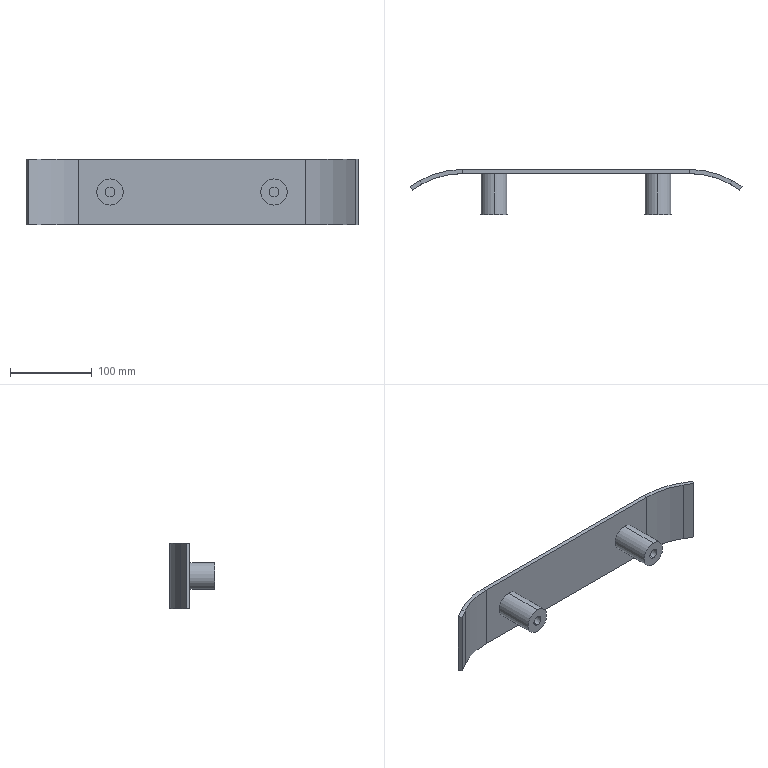Part | SolidWorks | features ICE 2, FlatPattern 1, SMBaseFlange 1, SheetMetal 1 | 1 solid | 34 faces | box 404.961 x 55 x 80 mm | volume 236837 mm3 | plane 22 | cylinder 12 | commonest cylinder face diameters 12 x4 32 x4 200 x2 210 x2
STEP:
#1=CARTESIAN_POINT('',(100.,-15.,6.));
#2=VERTEX_POINT('',#1);
#3=CARTESIAN_POINT('',(100.,-15.,-6.));
#4=VERTEX_POINT('',#3);
#5=CARTESIAN_POINT('',(100.,-15.,0.));
#6=DIRECTION('',(0.,-1.,0.));
#7=DIRECTION('',(0.,0.,-1.));
#8=AXIS2_PLACEMENT_3D('',#5,#6,#7);
#9=CIRCLE('',#8,6.);
#10=EDGE_CURVE('',#2,#4,#9,.T.);
#11=ORIENTED_EDGE('',*,*,#10,.F.);
#12=CARTESIAN_POINT('',(100.,-50.,6.));
#13=VERTEX_POINT('',#12);
#14=CARTESIAN_POINT('',(100.,-15.,6.));
#15=DIRECTION('',(0.,-1.,0.));
#16=VECTOR('',#15,1000.);
#17=LINE('',#14,#16);
#18=EDGE_CURVE('',#2,#13,#17,.T.);
#19=ORIENTED_EDGE('',*,*,#18,.T.);
#20=CARTESIAN_POINT('',(100.,-50.,-6.));
#21=VERTEX_POINT('',#20);
#22=CARTESIAN_POINT('',(100.,-50.,0.));
#23=DIRECTION('',(0.,-1.,0.));
#24=DIRECTION('',(0.,0.,-1.));
#25=AXIS2_PLACEMENT_3D('',#22,#23,#24);
#26=CIRCLE('',#25,6.);
#27=EDGE_CURVE('',#13,#21,#26,.T.);
#28=ORIENTED_EDGE('',*,*,#27,.T.);
#29=CARTESIAN_POINT('',(100.,-15.,-6.));
#30=DIRECTION('',(0.,-1.,0.));
#31=VECTOR('',#30,1000.);
#32=LINE('',#29,#31);
#33=EDGE_CURVE('',#4,#21,#32,.T.);
#34=ORIENTED_EDGE('',*,*,#33,.F.);
#35=EDGE_LOOP('',(#11,#19,#28,#34));
#36=FACE_OUTER_BOUND('',#35,.T.);
#37=CARTESIAN_POINT('',(100.,-15.,0.));
#38=DIRECTION('',(0.,-1.,0.));
#39=DIRECTION('',(0.,0.,-1.));
#40=AXIS2_PLACEMENT_3D('',#37,#38,#39);
#41=CYLINDRICAL_SURFACE('',#40,6.);
#42=ADVANCED_FACE('',(#36),#41,.F.);
#43=CARTESIAN_POINT('',(-100.,-15.,6.));
#44=VERTEX_POINT('',#43);
#45=CARTESIAN_POINT('',(-100.,-15.,-6.));
#46=VERTEX_POINT('',#45);
#47=CARTESIAN_POINT('',(-100.,-15.,0.));
#48=DIRECTION('',(0.,-1.,0.));
#49=DIRECTION('',(0.,0.,-1.));
#50=AXIS2_PLACEMENT_3D('',#47,#48,#49);
#51=CIRCLE('',#50,6.);
#52=EDGE_CURVE('',#44,#46,#51,.T.);
#53=ORIENTED_EDGE('',*,*,#52,.F.);
#54=CARTESIAN_POINT('',(-100.,-50.,6.));
#55=VERTEX_POINT('',#54);
#56=CARTESIAN_POINT('',(-100.,-15.,6.));
#57=DIRECTION('',(0.,-1.,0.));
#58=VECTOR('',#57,1000.);
#59=LINE('',#56,#58);
#60=EDGE_CURVE('',#44,#55,#59,.T.);
#61=ORIENTED_EDGE('',*,*,#60,.T.);
#62=CARTESIAN_POINT('',(-100.,-50.,-6.));
#63=VERTEX_POINT('',#62);
#64=CARTESIAN_POINT('',(-100.,-50.,0.));
#65=DIRECTION('',(0.,-1.,0.));
#66=DIRECTION('',(0.,0.,-1.));
#67=AXIS2_PLACEMENT_3D('',#64,#65,#66);
#68=CIRCLE('',#67,6.);
#69=EDGE_CURVE('',#55,#63,#68,.T.);
#70=ORIENTED_EDGE('',*,*,#69,.T.);
#71=CARTESIAN_POINT('',(-100.,-15.,-6.));
#72=DIRECTION('',(0.,-1.,0.));
#73=VECTOR('',#72,1000.);
#74=LINE('',#71,#73);
#75=EDGE_CURVE('',#46,#63,#74,.T.);
#76=ORIENTED_EDGE('',*,*,#75,.F.);
#77=EDGE_LOOP('',(#53,#61,#70,#76));
#78=FACE_OUTER_BOUND('',#77,.T.);
#79=CARTESIAN_POINT('',(-100.,-15.,0.));
#80=DIRECTION('',(0.,-1.,0.));
#81=DIRECTION('',(0.,0.,-1.));
#82=AXIS2_PLACEMENT_3D('',#79,#80,#81);
#83=CYLINDRICAL_SURFACE('',#82,6.);
#84=ADVANCED_FACE('',(#78),#83,.F.);
#85=CARTESIAN_POINT('',(-100.,-50.,-16.));
#86=VERTEX_POINT('',#85);
#87=CARTESIAN_POINT('',(-100.,-50.,16.));
#88=VERTEX_POINT('',#87);
#89=CARTESIAN_POINT('',(-100.,-50.,0.));
#90=DIRECTION('',(0.,-1.,0.));
#91=DIRECTION('',(0.,0.,-1.));
#92=AXIS2_PLACEMENT_3D('',#89,#90,#91);
#93=CIRCLE('',#92,16.);
#94=EDGE_CURVE('',#86,#88,#93,.T.);
#95=ORIENTED_EDGE('',*,*,#94,.F.);
#96=CARTESIAN_POINT('',(-100.,0.,-16.));
#97=VERTEX_POINT('',#96);
#98=CARTESIAN_POINT('',(-100.,-50.,-16.));
#99=DIRECTION('',(0.,1.,0.));
#100=VECTOR('',#99,1000.);
#101=LINE('',#98,#100);
#102=EDGE_CURVE('',#86,#97,#101,.T.);
#103=ORIENTED_EDGE('',*,*,#102,.T.);
#104=CARTESIAN_POINT('',(-100.,0.,16.));
#105=VERTEX_POINT('',#104);
#106=CARTESIAN_POINT('',(-100.,0.,0.));
#107=DIRECTION('',(0.,-1.,0.));
#108=DIRECTION('',(0.,0.,-1.));
#109=AXIS2_PLACEMENT_3D('',#106,#107,#108);
#110=CIRCLE('',#109,16.);
#111=EDGE_CURVE('',#97,#105,#110,.T.);
#112=ORIENTED_EDGE('',*,*,#111,.T.);
#113=CARTESIAN_POINT('',(-100.,-50.,16.));
#114=DIRECTION('',(0.,1.,0.));
#115=VECTOR('',#114,1000.);
#116=LINE('',#113,#115);
#117=EDGE_CURVE('',#88,#105,#116,.T.);
#118=ORIENTED_EDGE('',*,*,#117,.F.);
#119=EDGE_LOOP('',(#95,#103,#112,#118));
#120=FACE_OUTER_BOUND('',#119,.T.);
#121=CARTESIAN_POINT('',(-100.,-50.,0.));
#122=DIRECTION('',(0.,1.,0.));
#123=DIRECTION('',(0.,0.,1.));
#124=AXIS2_PLACEMENT_3D('',#121,#122,#123);
#125=CYLINDRICAL_SURFACE('',#124,16.);
#126=ADVANCED_FACE('',(#120),#125,.T.);
#127=CARTESIAN_POINT('',(100.,-50.,-16.));
#128=VERTEX_POINT('',#127);
#129=CARTESIAN_POINT('',(100.,-50.,16.));
#130=VERTEX_POINT('',#129);
#131=CARTESIAN_POINT('',(100.,-50.,0.));
#132=DIRECTION('',(0.,-1.,0.));
#133=DIRECTION('',(0.,0.,-1.));
#134=AXIS2_PLACEMENT_3D('',#131,#132,#133);
#135=CIRCLE('',#134,16.);
#136=EDGE_CURVE('',#128,#130,#135,.T.);
#137=ORIENTED_EDGE('',*,*,#136,.F.);
#138=CARTESIAN_POINT('',(100.,0.,-16.));
#139=VERTEX_POINT('',#138);
#140=CARTESIAN_POINT('',(100.,-50.,-16.));
#141=DIRECTION('',(0.,1.,0.));
#142=VECTOR('',#141,1000.);
#143=LINE('',#140,#142);
#144=EDGE_CURVE('',#128,#139,#143,.T.);
#145=ORIENTED_EDGE('',*,*,#144,.T.);
#146=CARTESIAN_POINT('',(100.,0.,16.));
#147=VERTEX_POINT('',#146);
#148=CARTESIAN_POINT('',(100.,0.,0.));
#149=DIRECTION('',(0.,-1.,0.));
#150=DIRECTION('',(0.,0.,-1.));
#151=AXIS2_PLACEMENT_3D('',#148,#149,#150);
#152=CIRCLE('',#151,16.);
#153=EDGE_CURVE('',#139,#147,#152,.T.);
#154=ORIENTED_EDGE('',*,*,#153,.T.);
#155=CARTESIAN_POINT('',(100.,-50.,16.));
#156=DIRECTION('',(0.,1.,0.));
#157=VECTOR('',#156,1000.);
#158=LINE('',#155,#157);
#159=EDGE_CURVE('',#130,#147,#158,.T.);
#160=ORIENTED_EDGE('',*,*,#159,.F.);
#161=EDGE_LOOP('',(#137,#145,#154,#160));
#162=FACE_OUTER_BOUND('',#161,.T.);
#163=CARTESIAN_POINT('',(100.,-50.,0.));
#164=DIRECTION('',(0.,1.,0.));
#165=DIRECTION('',(0.,0.,1.));
#166=AXIS2_PLACEMENT_3D('',#163,#164,#165);
#167=CYLINDRICAL_SURFACE('',#166,16.);
#168=ADVANCED_FACE('',(#162),#167,.T.);
#169=CARTESIAN_POINT('',(138.444,0.,40.));
#170=VERTEX_POINT('',#169);
#171=CARTESIAN_POINT('',(138.444,5.,40.));
#172=VERTEX_POINT('',#171);
#173=CARTESIAN_POINT('',(138.444,0.,40.));
#174=DIRECTION('',(0.,1.,0.));
#175=VECTOR('',#174,1000.);
#176=LINE('',#173,#175);
#177=EDGE_CURVE('',#170,#172,#176,.T.);
#178=ORIENTED_EDGE('',*,*,#177,.F.);
#179=CARTESIAN_POINT('',(188.057,-13.176,40.));
#180=VERTEX_POINT('',#179);
#181=CARTESIAN_POINT('',(138.444,-100.,40.));
#182=DIRECTION('',(0.,0.,1.));
#183=DIRECTION('',(-1.,0.,0.));
#184=AXIS2_PLACEMENT_3D('',#181,#182,#183);
#185=CIRCLE('',#184,100.);
#186=EDGE_CURVE('',#180,#170,#185,.T.);
#187=ORIENTED_EDGE('',*,*,#186,.F.);
#188=CARTESIAN_POINT('',(190.538,-8.834,40.));
#189=VERTEX_POINT('',#188);
#190=CARTESIAN_POINT('',(190.538,-8.834,40.));
#191=DIRECTION('',(-0.4961,-0.8682,0.));
#192=VECTOR('',#191,1000.);
#193=LINE('',#190,#192);
#194=EDGE_CURVE('',#189,#180,#193,.T.);
#195=ORIENTED_EDGE('',*,*,#194,.F.);
#196=CARTESIAN_POINT('',(138.444,-100.,40.));
#197=DIRECTION('',(0.,0.,1.));
#198=DIRECTION('',(1.,0.,0.));
#199=AXIS2_PLACEMENT_3D('',#196,#197,#198);
#200=CIRCLE('',#199,105.);
#201=EDGE_CURVE('',#189,#172,#200,.T.);
#202=ORIENTED_EDGE('',*,*,#201,.T.);
#203=EDGE_LOOP('',(#178,#187,#195,#202));
#204=FACE_OUTER_BOUND('',#203,.T.);
#205=CARTESIAN_POINT('',(138.444,0.,40.));
#206=DIRECTION('',(0.,0.,1.));
#207=DIRECTION('',(1.,0.,0.));
#208=AXIS2_PLACEMENT_3D('',#205,#206,#207);
#209=PLANE('',#208);
#210=ADVANCED_FACE('',(#204),#209,.T.);
#211=CARTESIAN_POINT('',(-138.444,0.,40.));
#212=VERTEX_POINT('',#211);
#213=CARTESIAN_POINT('',(-165.,0.,40.));
#214=DIRECTION('',(-1.,0.,0.));
#215=VECTOR('',#214,1000.);
#216=LINE('',#213,#215);
#217=EDGE_CURVE('',#170,#212,#216,.T.);
#218=ORIENTED_EDGE('',*,*,#217,.F.);
#219=ORIENTED_EDGE('',*,*,#177,.T.);
#220=CARTESIAN_POINT('',(-138.444,5.,40.));
#221=VERTEX_POINT('',#220);
#222=CARTESIAN_POINT('',(-165.,5.,40.));
#223=DIRECTION('',(-1.,0.,0.));
#224=VECTOR('',#223,1000.);
#225=LINE('',#222,#224);
#226=EDGE_CURVE('',#172,#221,#225,.T.);
#227=ORIENTED_EDGE('',*,*,#226,.T.);
#228=CARTESIAN_POINT('',(-138.444,5.,40.));
#229=DIRECTION('',(0.,-1.,0.));
#230=VECTOR('',#229,1000.);
#231=LINE('',#228,#230);
#232=EDGE_CURVE('',#221,#212,#231,.T.);
#233=ORIENTED_EDGE('',*,*,#232,.T.);
#234=EDGE_LOOP('',(#218,#219,#227,#233));
#235=FACE_OUTER_BOUND('',#234,.T.);
#236=CARTESIAN_POINT('',(190.538,-8.834,40.));
#237=DIRECTION('',(0.,0.,1.));
#238=DIRECTION('',(1.,0.,0.));
#239=AXIS2_PLACEMENT_3D('',#236,#237,#238);
#240=PLANE('',#239);
#241=ADVANCED_FACE('',(#235),#240,.T.);
#242=CARTESIAN_POINT('',(188.057,-13.176,-40.));
#243=VERTEX_POINT('',#242);
#244=CARTESIAN_POINT('',(190.538,-8.834,-40.));
#245=VERTEX_POINT('',#244);
#246=CARTESIAN_POINT('',(188.057,-13.176,-40.));
#247=DIRECTION('',(0.4961,0.8682,0.));
#248=VECTOR('',#247,1000.);
#249=LINE('',#246,#248);
#250=EDGE_CURVE('',#243,#245,#249,.T.);
#251=ORIENTED_EDGE('',*,*,#250,.F.);
#252=CARTESIAN_POINT('',(138.444,0.,-40.));
#253=VERTEX_POINT('',#252);
#254=CARTESIAN_POINT('',(138.444,-100.,-40.));
#255=DIRECTION('',(0.,0.,1.));
#256=DIRECTION('',(-1.,0.,0.));
#257=AXIS2_PLACEMENT_3D('',#254,#255,#256);
#258=CIRCLE('',#257,100.);
#259=EDGE_CURVE('',#243,#253,#258,.T.);
#260=ORIENTED_EDGE('',*,*,#259,.T.);
#261=CARTESIAN_POINT('',(138.444,5.,-40.));
#262=VERTEX_POINT('',#261);
#263=CARTESIAN_POINT('',(138.444,5.,-40.));
#264=DIRECTION('',(0.,-1.,0.));
#265=VECTOR('',#264,1000.);
#266=LINE('',#263,#265);
#267=EDGE_CURVE('',#262,#253,#266,.T.);
#268=ORIENTED_EDGE('',*,*,#267,.F.);
#269=CARTESIAN_POINT('',(138.444,-100.,-40.));
#270=DIRECTION('',(0.,0.,1.));
#271=DIRECTION('',(1.,0.,0.));
#272=AXIS2_PLACEMENT_3D('',#269,#270,#271);
#273=CIRCLE('',#272,105.);
#274=EDGE_CURVE('',#245,#262,#273,.T.);
#275=ORIENTED_EDGE('',*,*,#274,.F.);
#276=EDGE_LOOP('',(#251,#260,#268,#275));
#277=FACE_OUTER_BOUND('',#276,.T.);
#278=CARTESIAN_POINT('',(188.057,-13.176,-40.));
#279=DIRECTION('',(0.,0.,-1.));
#280=DIRECTION('',(-1.,0.,0.));
#281=AXIS2_PLACEMENT_3D('',#278,#279,#280);
#282=PLANE('',#281);
#283=ADVANCED_FACE('',(#277),#282,.T.);
#284=CARTESIAN_POINT('',(200.,-20.,-40.));
#285=VERTEX_POINT('',#284);
#286=CARTESIAN_POINT('',(165.,0.,-40.));
#287=DIRECTION('',(-0.8682,0.4961,0.));
#288=VECTOR('',#287,1000.);
#289=LINE('',#286,#288);
#290=EDGE_CURVE('',#285,#243,#289,.T.);
#291=ORIENTED_EDGE('',*,*,#290,.T.);
#292=ORIENTED_EDGE('',*,*,#250,.T.);
#293=CARTESIAN_POINT('',(202.481,-15.659,-40.));
#294=VERTEX_POINT('',#293);
#295=CARTESIAN_POINT('',(167.481,4.341,-40.));
#296=DIRECTION('',(-0.8682,0.4961,0.));
#297=VECTOR('',#296,1000.);
#298=LINE('',#295,#297);
#299=EDGE_CURVE('',#294,#245,#298,.T.);
#300=ORIENTED_EDGE('',*,*,#299,.F.);
#301=CARTESIAN_POINT('',(202.481,-15.659,-40.));
#302=DIRECTION('',(-0.4961,-0.8682,0.));
#303=VECTOR('',#302,1000.);
#304=LINE('',#301,#303);
#305=EDGE_CURVE('',#294,#285,#304,.T.);
#306=ORIENTED_EDGE('',*,*,#305,.T.);
#307=EDGE_LOOP('',(#291,#292,#300,#306));
#308=FACE_OUTER_BOUND('',#307,.T.);
#309=CARTESIAN_POINT('',(138.444,5.,-40.));
#310=DIRECTION('',(0.,0.,-1.));
#311=DIRECTION('',(-1.,0.,0.));
#312=AXIS2_PLACEMENT_3D('',#309,#310,#311);
#313=PLANE('',#312);
#314=ADVANCED_FACE('',(#308),#313,.T.);
#315=CARTESIAN_POINT('',(-188.057,-13.176,40.));
#316=VERTEX_POINT('',#315);
#317=CARTESIAN_POINT('',(-190.538,-8.834,40.));
#318=VERTEX_POINT('',#317);
#319=CARTESIAN_POINT('',(-188.057,-13.176,40.));
#320=DIRECTION('',(-0.4961,0.8682,0.));
#321=VECTOR('',#320,1000.);
#322=LINE('',#319,#321);
#323=EDGE_CURVE('',#316,#318,#322,.T.);
#324=ORIENTED_EDGE('',*,*,#323,.F.);
#325=CARTESIAN_POINT('',(-138.444,-100.,40.));
#326=DIRECTION('',(0.,0.,1.));
#327=DIRECTION('',(-1.,0.,0.));
#328=AXIS2_PLACEMENT_3D('',#325,#326,#327);
#329=CIRCLE('',#328,100.);
#330=EDGE_CURVE('',#212,#316,#329,.T.);
#331=ORIENTED_EDGE('',*,*,#330,.F.);
#332=ORIENTED_EDGE('',*,*,#232,.F.);
#333=CARTESIAN_POINT('',(-138.444,-100.,40.));
#334=DIRECTION('',(0.,0.,1.));
#335=DIRECTION('',(1.,0.,0.));
#336=AXIS2_PLACEMENT_3D('',#333,#334,#335);
#337=CIRCLE('',#336,105.);
#338=EDGE_CURVE('',#221,#318,#337,.T.);
#339=ORIENTED_EDGE('',*,*,#338,.T.);
#340=EDGE_LOOP('',(#324,#331,#332,#339));
#341=FACE_OUTER_BOUND('',#340,.T.);
#342=CARTESIAN_POINT('',(-188.057,-13.176,40.));
#343=DIRECTION('',(0.,0.,1.));
#344=DIRECTION('',(1.,0.,0.));
#345=AXIS2_PLACEMENT_3D('',#342,#343,#344);
#346=PLANE('',#345);
#347=ADVANCED_FACE('',(#341),#346,.T.);
#348=CARTESIAN_POINT('',(-200.,-20.,40.));
#349=VERTEX_POINT('',#348);
#350=CARTESIAN_POINT('',(-165.,0.,40.));
#351=DIRECTION('',(-0.8682,-0.4961,0.));
#352=VECTOR('',#351,1000.);
#353=LINE('',#350,#352);
#354=EDGE_CURVE('',#316,#349,#353,.T.);
#355=ORIENTED_EDGE('',*,*,#354,.F.);
#356=ORIENTED_EDGE('',*,*,#323,.T.);
#357=CARTESIAN_POINT('',(-202.481,-15.659,40.));
#358=VERTEX_POINT('',#357);
#359=CARTESIAN_POINT('',(-167.481,4.341,40.));
#360=DIRECTION('',(-0.8682,-0.4961,0.));
#361=VECTOR('',#360,1000.);
#362=LINE('',#359,#361);
#363=EDGE_CURVE('',#318,#358,#362,.T.);
#364=ORIENTED_EDGE('',*,*,#363,.T.);
#365=CARTESIAN_POINT('',(-200.,-20.,40.));
#366=DIRECTION('',(-0.4961,0.8682,0.));
#367=VECTOR('',#366,1000.);
#368=LINE('',#365,#367);
#369=EDGE_CURVE('',#349,#358,#368,.T.);
#370=ORIENTED_EDGE('',*,*,#369,.F.);
#371=EDGE_LOOP('',(#355,#356,#364,#370));
#372=FACE_OUTER_BOUND('',#371,.T.);
#373=CARTESIAN_POINT('',(-138.444,5.,40.));
#374=DIRECTION('',(0.,0.,1.));
#375=DIRECTION('',(1.,0.,0.));
#376=AXIS2_PLACEMENT_3D('',#373,#374,#375);
#377=PLANE('',#376);
#378=ADVANCED_FACE('',(#372),#377,.T.);
#379=CARTESIAN_POINT('',(-138.444,0.,-40.));
#380=VERTEX_POINT('',#379);
#381=CARTESIAN_POINT('',(-138.444,5.,-40.));
#382=VERTEX_POINT('',#381);
#383=CARTESIAN_POINT('',(-138.444,0.,-40.));
#384=DIRECTION('',(0.,1.,0.));
#385=VECTOR('',#384,1000.);
#386=LINE('',#383,#385);
#387=EDGE_CURVE('',#380,#382,#386,.T.);
#388=ORIENTED_EDGE('',*,*,#387,.F.);
#389=CARTESIAN_POINT('',(-188.057,-13.176,-40.));
#390=VERTEX_POINT('',#389);
#391=CARTESIAN_POINT('',(-138.444,-100.,-40.));
#392=DIRECTION('',(0.,0.,1.));
#393=DIRECTION('',(-1.,0.,0.));
#394=AXIS2_PLACEMENT_3D('',#391,#392,#393);
#395=CIRCLE('',#394,100.);
#396=EDGE_CURVE('',#380,#390,#395,.T.);
#397=ORIENTED_EDGE('',*,*,#396,.T.);
#398=CARTESIAN_POINT('',(-190.538,-8.834,-40.));
#399=VERTEX_POINT('',#398);
#400=CARTESIAN_POINT('',(-190.538,-8.834,-40.));
#401=DIRECTION('',(0.4961,-0.8682,0.));
#402=VECTOR('',#401,1000.);
#403=LINE('',#400,#402);
#404=EDGE_CURVE('',#399,#390,#403,.T.);
#405=ORIENTED_EDGE('',*,*,#404,.F.);
#406=CARTESIAN_POINT('',(-138.444,-100.,-40.));
#407=DIRECTION('',(0.,0.,1.));
#408=DIRECTION('',(1.,0.,0.));
#409=AXIS2_PLACEMENT_3D('',#406,#407,#408);
#410=CIRCLE('',#409,105.);
#411=EDGE_CURVE('',#382,#399,#410,.T.);
#412=ORIENTED_EDGE('',*,*,#411,.F.);
#413=EDGE_LOOP('',(#388,#397,#405,#412));
#414=FACE_OUTER_BOUND('',#413,.T.);
#415=CARTESIAN_POINT('',(-138.444,0.,-40.));
#416=DIRECTION('',(0.,0.,-1.));
#417=DIRECTION('',(-1.,0.,0.));
#418=AXIS2_PLACEMENT_3D('',#415,#416,#417);
#419=PLANE('',#418);
#420=ADVANCED_FACE('',(#414),#419,.T.);
#421=CARTESIAN_POINT('',(-165.,0.,-40.));
#422=DIRECTION('',(-1.,0.,0.));
#423=VECTOR('',#422,1000.);
#424=LINE('',#421,#423);
#425=EDGE_CURVE('',#253,#380,#424,.T.);
#426=ORIENTED_EDGE('',*,*,#425,.T.);
#427=ORIENTED_EDGE('',*,*,#387,.T.);
#428=CARTESIAN_POINT('',(-165.,5.,-40.));
#429=DIRECTION('',(-1.,0.,0.));
#430=VECTOR('',#429,1000.);
#431=LINE('',#428,#430);
#432=EDGE_CURVE('',#262,#382,#431,.T.);
#433=ORIENTED_EDGE('',*,*,#432,.F.);
#434=ORIENTED_EDGE('',*,*,#267,.T.);
#435=EDGE_LOOP('',(#426,#427,#433,#434));
#436=FACE_OUTER_BOUND('',#435,.T.);
#437=CARTESIAN_POINT('',(-190.538,-8.834,-40.));
#438=DIRECTION('',(0.,0.,-1.));
#439=DIRECTION('',(-1.,0.,0.));
#440=AXIS2_PLACEMENT_3D('',#437,#438,#439);
#441=PLANE('',#440);
#442=ADVANCED_FACE('',(#436),#441,.T.);
#443=CARTESIAN_POINT('',(-202.481,-15.659,-40.));
#444=VERTEX_POINT('',#443);
#445=CARTESIAN_POINT('',(-167.481,4.341,-40.));
#446=DIRECTION('',(-0.8682,-0.4961,0.));
#447=VECTOR('',#446,1000.);
#448=LINE('',#445,#447);
#449=EDGE_CURVE('',#399,#444,#448,.T.);
#450=ORIENTED_EDGE('',*,*,#449,.T.);
#451=CARTESIAN_POINT('',(-202.481,-15.659,40.));
#452=DIRECTION('',(0.,0.,-1.));
#453=VECTOR('',#452,1000.);
#454=LINE('',#451,#453);
#455=EDGE_CURVE('',#358,#444,#454,.T.);
#456=ORIENTED_EDGE('',*,*,#455,.F.);
#457=ORIENTED_EDGE('',*,*,#363,.F.);
#458=CARTESIAN_POINT('',(-190.538,-8.834,40.));
#459=DIRECTION('',(0.,0.,-1.));
#460=VECTOR('',#459,1000.);
#461=LINE('',#458,#460);
#462=EDGE_CURVE('',#318,#399,#461,.T.);
#463=ORIENTED_EDGE('',*,*,#462,.T.);
#464=EDGE_LOOP('',(#450,#456,#457,#463));
#465=FACE_OUTER_BOUND('',#464,.T.);
#466=CARTESIAN_POINT('',(-167.481,4.341,40.));
#467=DIRECTION('',(0.4961,-0.8682,0.));
#468=DIRECTION('',(0.8682,0.4961,0.));
#469=AXIS2_PLACEMENT_3D('',#466,#467,#468);
#470=PLANE('',#469);
#471=ADVANCED_FACE('',(#465),#470,.F.);
#472=CARTESIAN_POINT('',(-200.,-20.,-40.));
#473=VERTEX_POINT('',#472);
#474=CARTESIAN_POINT('',(-200.,-20.,-40.));
#475=DIRECTION('',(-0.4961,0.8682,0.));
#476=VECTOR('',#475,1000.);
#477=LINE('',#474,#476);
#478=EDGE_CURVE('',#473,#444,#477,.T.);
#479=ORIENTED_EDGE('',*,*,#478,.F.);
#480=CARTESIAN_POINT('',(-200.,-20.,40.));
#481=DIRECTION('',(0.,0.,-1.));
#482=VECTOR('',#481,1000.);
#483=LINE('',#480,#482);
#484=EDGE_CURVE('',#349,#473,#483,.T.);
#485=ORIENTED_EDGE('',*,*,#484,.F.);
#486=ORIENTED_EDGE('',*,*,#369,.T.);
#487=ORIENTED_EDGE('',*,*,#455,.T.);
#488=EDGE_LOOP('',(#479,#485,#486,#487));
#489=FACE_OUTER_BOUND('',#488,.T.);
#490=CARTESIAN_POINT('',(-200.,-20.,40.));
#491=DIRECTION('',(-0.8682,-0.4961,0.));
#492=DIRECTION('',(0.4961,-0.8682,0.));
#493=AXIS2_PLACEMENT_3D('',#490,#491,#492);
#494=PLANE('',#493);
#495=ADVANCED_FACE('',(#489),#494,.T.);
#496=CARTESIAN_POINT('',(-165.,0.,-40.));
#497=DIRECTION('',(-0.8682,-0.4961,0.));
#498=VECTOR('',#497,1000.);
#499=LINE('',#496,#498);
#500=EDGE_CURVE('',#390,#473,#499,.T.);
#501=ORIENTED_EDGE('',*,*,#500,.F.);
#502=CARTESIAN_POINT('',(-188.057,-13.176,40.));
#503=DIRECTION('',(0.,0.,-1.));
#504=VECTOR('',#503,1000.);
#505=LINE('',#502,#504);
#506=EDGE_CURVE('',#316,#390,#505,.T.);
#507=ORIENTED_EDGE('',*,*,#506,.F.);
#508=ORIENTED_EDGE('',*,*,#354,.T.);
#509=ORIENTED_EDGE('',*,*,#484,.T.);
#510=EDGE_LOOP('',(#501,#507,#508,#509));
#511=FACE_OUTER_BOUND('',#510,.T.);
#512=CARTESIAN_POINT('',(-165.,0.,40.));
#513=DIRECTION('',(0.4961,-0.8682,0.));
#514=DIRECTION('',(0.8682,0.4961,0.));
#515=AXIS2_PLACEMENT_3D('',#512,#513,#514);
#516=PLANE('',#515);
#517=ADVANCED_FACE('',(#511),#516,.T.);
#518=ORIENTED_EDGE('',*,*,#396,.F.);
#519=CARTESIAN_POINT('',(-138.444,0.,40.));
#520=DIRECTION('',(0.,0.,-1.));
#521=VECTOR('',#520,1000.);
#522=LINE('',#519,#521);
#523=EDGE_CURVE('',#212,#380,#522,.T.);
#524=ORIENTED_EDGE('',*,*,#523,.F.);
#525=ORIENTED_EDGE('',*,*,#330,.T.);
#526=ORIENTED_EDGE('',*,*,#506,.T.);
#527=EDGE_LOOP('',(#518,#524,#525,#526));
#528=FACE_OUTER_BOUND('',#527,.T.);
#529=CARTESIAN_POINT('',(-138.444,-100.,40.));
#530=DIRECTION('',(0.,0.,-1.));
#531=DIRECTION('',(-1.,0.,0.));
#532=AXIS2_PLACEMENT_3D('',#529,#530,#531);
#533=CYLINDRICAL_SURFACE('',#532,100.);
#534=ADVANCED_FACE('',(#528),#533,.F.);
#535=CARTESIAN_POINT('',(-100.,0.,0.));
#536=DIRECTION('',(0.,-1.,0.));
#537=DIRECTION('',(0.,0.,-1.));
#538=AXIS2_PLACEMENT_3D('',#535,#536,#537);
#539=CIRCLE('',#538,16.);
#540=EDGE_CURVE('',#105,#97,#539,.T.);
#541=ORIENTED_EDGE('',*,*,#540,.F.);
#542=ORIENTED_EDGE('',*,*,#111,.F.);
#543=EDGE_LOOP('',(#541,#542));
#544=FACE_BOUND('',#543,.T.);
#545=CARTESIAN_POINT('',(100.,0.,0.));
#546=DIRECTION('',(0.,-1.,0.));
#547=DIRECTION('',(0.,0.,-1.));
#548=AXIS2_PLACEMENT_3D('',#545,#546,#547);
#549=CIRCLE('',#548,16.);
#550=EDGE_CURVE('',#147,#139,#549,.T.);
#551=ORIENTED_EDGE('',*,*,#550,.F.);
#552=ORIENTED_EDGE('',*,*,#153,.F.);
#553=EDGE_LOOP('',(#551,#552));
#554=FACE_BOUND('',#553,.T.);
#555=ORIENTED_EDGE('',*,*,#425,.F.);
#556=CARTESIAN_POINT('',(138.444,0.,40.));
#557=DIRECTION('',(0.,0.,-1.));
#558=VECTOR('',#557,1000.);
#559=LINE('',#556,#558);
#560=EDGE_CURVE('',#170,#253,#559,.T.);
#561=ORIENTED_EDGE('',*,*,#560,.F.);
#562=ORIENTED_EDGE('',*,*,#217,.T.);
#563=ORIENTED_EDGE('',*,*,#523,.T.);
#564=EDGE_LOOP('',(#555,#561,#562,#563));
#565=FACE_OUTER_BOUND('',#564,.T.);
#566=CARTESIAN_POINT('',(-165.,0.,40.));
#567=DIRECTION('',(0.,-1.,0.));
#568=DIRECTION('',(0.,0.,-1.));
#569=AXIS2_PLACEMENT_3D('',#566,#567,#568);
#570=PLANE('',#569);
#571=ADVANCED_FACE('',(#544,#554,#565),#570,.T.);
#572=ORIENTED_EDGE('',*,*,#259,.F.);
#573=CARTESIAN_POINT('',(188.057,-13.176,40.));
#574=DIRECTION('',(0.,0.,-1.));
#575=VECTOR('',#574,1000.);
#576=LINE('',#573,#575);
#577=EDGE_CURVE('',#180,#243,#576,.T.);
#578=ORIENTED_EDGE('',*,*,#577,.F.);
#579=ORIENTED_EDGE('',*,*,#186,.T.);
#580=ORIENTED_EDGE('',*,*,#560,.T.);
#581=EDGE_LOOP('',(#572,#578,#579,#580));
#582=FACE_OUTER_BOUND('',#581,.T.);
#583=CARTESIAN_POINT('',(138.444,-100.,40.));
#584=DIRECTION('',(0.,0.,-1.));
#585=DIRECTION('',(-1.,0.,0.));
#586=AXIS2_PLACEMENT_3D('',#583,#584,#585);
#587=CYLINDRICAL_SURFACE('',#586,100.);
#588=ADVANCED_FACE('',(#582),#587,.F.);
#589=ORIENTED_EDGE('',*,*,#290,.F.);
#590=CARTESIAN_POINT('',(200.,-20.,40.));
#591=VERTEX_POINT('',#590);
#592=CARTESIAN_POINT('',(200.,-20.,40.));
#593=DIRECTION('',(0.,0.,-1.));
#594=VECTOR('',#593,1000.);
#595=LINE('',#592,#594);
#596=EDGE_CURVE('',#591,#285,#595,.T.);
#597=ORIENTED_EDGE('',*,*,#596,.F.);
#598=CARTESIAN_POINT('',(165.,0.,40.));
#599=DIRECTION('',(-0.8682,0.4961,0.));
#600=VECTOR('',#599,1000.);
#601=LINE('',#598,#600);
#602=EDGE_CURVE('',#591,#180,#601,.T.);
#603=ORIENTED_EDGE('',*,*,#602,.T.);
#604=ORIENTED_EDGE('',*,*,#577,.T.);
#605=EDGE_LOOP('',(#589,#597,#603,#604));
#606=FACE_OUTER_BOUND('',#605,.T.);
#607=CARTESIAN_POINT('',(165.,0.,40.));
#608=DIRECTION('',(-0.4961,-0.8682,0.));
#609=DIRECTION('',(0.8682,-0.4961,0.));
#610=AXIS2_PLACEMENT_3D('',#607,#608,#609);
#611=PLANE('',#610);
#612=ADVANCED_FACE('',(#606),#611,.T.);
#613=ORIENTED_EDGE('',*,*,#305,.F.);
#614=CARTESIAN_POINT('',(202.481,-15.659,40.));
#615=VERTEX_POINT('',#614);
#616=CARTESIAN_POINT('',(202.481,-15.659,40.));
#617=DIRECTION('',(0.,0.,-1.));
#618=VECTOR('',#617,1000.);
#619=LINE('',#616,#618);
#620=EDGE_CURVE('',#615,#294,#619,.T.);
#621=ORIENTED_EDGE('',*,*,#620,.F.);
#622=CARTESIAN_POINT('',(202.481,-15.659,40.));
#623=DIRECTION('',(-0.4961,-0.8682,0.));
#624=VECTOR('',#623,1000.);
#625=LINE('',#622,#624);
#626=EDGE_CURVE('',#615,#591,#625,.T.);
#627=ORIENTED_EDGE('',*,*,#626,.T.);
#628=ORIENTED_EDGE('',*,*,#596,.T.);
#629=EDGE_LOOP('',(#613,#621,#627,#628));
#630=FACE_OUTER_BOUND('',#629,.T.);
#631=CARTESIAN_POINT('',(202.481,-15.659,40.));
#632=DIRECTION('',(0.8682,-0.4961,0.));
#633=DIRECTION('',(0.4961,0.8682,0.));
#634=AXIS2_PLACEMENT_3D('',#631,#632,#633);
#635=PLANE('',#634);
#636=ADVANCED_FACE('',(#630),#635,.T.);
#637=ORIENTED_EDGE('',*,*,#299,.T.);
#638=CARTESIAN_POINT('',(190.538,-8.834,40.));
#639=DIRECTION('',(0.,0.,-1.));
#640=VECTOR('',#639,1000.);
#641=LINE('',#638,#640);
#642=EDGE_CURVE('',#189,#245,#641,.T.);
#643=ORIENTED_EDGE('',*,*,#642,.F.);
#644=CARTESIAN_POINT('',(167.481,4.341,40.));
#645=DIRECTION('',(-0.8682,0.4961,0.));
#646=VECTOR('',#645,1000.);
#647=LINE('',#644,#646);
#648=EDGE_CURVE('',#615,#189,#647,.T.);
#649=ORIENTED_EDGE('',*,*,#648,.F.);
#650=ORIENTED_EDGE('',*,*,#620,.T.);
#651=EDGE_LOOP('',(#637,#643,#649,#650));
#652=FACE_OUTER_BOUND('',#651,.T.);
#653=CARTESIAN_POINT('',(167.481,4.341,40.));
#654=DIRECTION('',(-0.4961,-0.8682,0.));
#655=DIRECTION('',(0.8682,-0.4961,0.));
#656=AXIS2_PLACEMENT_3D('',#653,#654,#655);
#657=PLANE('',#656);
#658=ADVANCED_FACE('',(#652),#657,.F.);
#659=ORIENTED_EDGE('',*,*,#274,.T.);
#660=CARTESIAN_POINT('',(138.444,5.,40.));
#661=DIRECTION('',(0.,0.,-1.));
#662=VECTOR('',#661,1000.);
#663=LINE('',#660,#662);
#664=EDGE_CURVE('',#172,#262,#663,.T.);
#665=ORIENTED_EDGE('',*,*,#664,.F.);
#666=ORIENTED_EDGE('',*,*,#201,.F.);
#667=ORIENTED_EDGE('',*,*,#642,.T.);
#668=EDGE_LOOP('',(#659,#665,#666,#667));
#669=FACE_OUTER_BOUND('',#668,.T.);
#670=CARTESIAN_POINT('',(138.444,-100.,40.));
#671=DIRECTION('',(0.,0.,-1.));
#672=DIRECTION('',(-1.,0.,0.));
#673=AXIS2_PLACEMENT_3D('',#670,#671,#672);
#674=CYLINDRICAL_SURFACE('',#673,105.);
#675=ADVANCED_FACE('',(#669),#674,.T.);
#676=ORIENTED_EDGE('',*,*,#432,.T.);
#677=CARTESIAN_POINT('',(-138.444,5.,40.));
#678=DIRECTION('',(0.,0.,-1.));
#679=VECTOR('',#678,1000.);
#680=LINE('',#677,#679);
#681=EDGE_CURVE('',#221,#382,#680,.T.);
#682=ORIENTED_EDGE('',*,*,#681,.F.);
#683=ORIENTED_EDGE('',*,*,#226,.F.);
#684=ORIENTED_EDGE('',*,*,#664,.T.);
#685=EDGE_LOOP('',(#676,#682,#683,#684));
#686=FACE_OUTER_BOUND('',#685,.T.);
#687=CARTESIAN_POINT('',(-165.,5.,40.));
#688=DIRECTION('',(0.,-1.,0.));
#689=DIRECTION('',(0.,0.,-1.));
#690=AXIS2_PLACEMENT_3D('',#687,#688,#689);
#691=PLANE('',#690);
#692=ADVANCED_FACE('',(#686),#691,.F.);
#693=ORIENTED_EDGE('',*,*,#411,.T.);
#694=ORIENTED_EDGE('',*,*,#462,.F.);
#695=ORIENTED_EDGE('',*,*,#338,.F.);
#696=ORIENTED_EDGE('',*,*,#681,.T.);
#697=EDGE_LOOP('',(#693,#694,#695,#696));
#698=FACE_OUTER_BOUND('',#697,.T.);
#699=CARTESIAN_POINT('',(-138.444,-100.,40.));
#700=DIRECTION('',(0.,0.,-1.));
#701=DIRECTION('',(-1.,0.,0.));
#702=AXIS2_PLACEMENT_3D('',#699,#700,#701);
#703=CYLINDRICAL_SURFACE('',#702,105.);
#704=ADVANCED_FACE('',(#698),#703,.T.);
#705=ORIENTED_EDGE('',*,*,#648,.T.);
#706=ORIENTED_EDGE('',*,*,#194,.T.);
#707=ORIENTED_EDGE('',*,*,#602,.F.);
#708=ORIENTED_EDGE('',*,*,#626,.F.);
#709=EDGE_LOOP('',(#705,#706,#707,#708));
#710=FACE_OUTER_BOUND('',#709,.T.);
#711=CARTESIAN_POINT('',(-138.444,-100.,40.));
#712=DIRECTION('',(0.,0.,-1.));
#713=DIRECTION('',(-1.,0.,0.));
#714=AXIS2_PLACEMENT_3D('',#711,#712,#713);
#715=PLANE('',#714);
#716=ADVANCED_FACE('',(#710),#715,.F.);
#717=ORIENTED_EDGE('',*,*,#449,.F.);
#718=ORIENTED_EDGE('',*,*,#404,.T.);
#719=ORIENTED_EDGE('',*,*,#500,.T.);
#720=ORIENTED_EDGE('',*,*,#478,.T.);
#721=EDGE_LOOP('',(#717,#718,#719,#720));
#722=FACE_OUTER_BOUND('',#721,.T.);
#723=CARTESIAN_POINT('',(-138.444,-100.,-40.));
#724=DIRECTION('',(0.,0.,-1.));
#725=DIRECTION('',(-1.,0.,0.));
#726=AXIS2_PLACEMENT_3D('',#723,#724,#725);
#727=PLANE('',#726);
#728=ADVANCED_FACE('',(#722),#727,.T.);
#729=ORIENTED_EDGE('',*,*,#144,.F.);
#730=CARTESIAN_POINT('',(100.,-50.,0.));
#731=DIRECTION('',(0.,-1.,0.));
#732=DIRECTION('',(0.,0.,-1.));
#733=AXIS2_PLACEMENT_3D('',#730,#731,#732);
#734=CIRCLE('',#733,16.);
#735=EDGE_CURVE('',#130,#128,#734,.T.);
#736=ORIENTED_EDGE('',*,*,#735,.F.);
#737=ORIENTED_EDGE('',*,*,#159,.T.);
#738=ORIENTED_EDGE('',*,*,#550,.T.);
#739=EDGE_LOOP('',(#729,#736,#737,#738));
#740=FACE_OUTER_BOUND('',#739,.T.);
#741=CARTESIAN_POINT('',(100.,-50.,0.));
#742=DIRECTION('',(0.,1.,0.));
#743=DIRECTION('',(0.,0.,1.));
#744=AXIS2_PLACEMENT_3D('',#741,#742,#743);
#745=CYLINDRICAL_SURFACE('',#744,16.);
#746=ADVANCED_FACE('',(#740),#745,.T.);
#747=CARTESIAN_POINT('',(100.,-50.,0.));
#748=DIRECTION('',(0.,-1.,0.));
#749=DIRECTION('',(0.,0.,-1.));
#750=AXIS2_PLACEMENT_3D('',#747,#748,#749);
#751=CIRCLE('',#750,6.);
#752=EDGE_CURVE('',#21,#13,#751,.T.);
#753=ORIENTED_EDGE('',*,*,#752,.F.);
#754=ORIENTED_EDGE('',*,*,#27,.F.);
#755=EDGE_LOOP('',(#753,#754));
#756=FACE_BOUND('',#755,.T.);
#757=ORIENTED_EDGE('',*,*,#735,.T.);
#758=ORIENTED_EDGE('',*,*,#136,.T.);
#759=EDGE_LOOP('',(#757,#758));
#760=FACE_OUTER_BOUND('',#759,.T.);
#761=CARTESIAN_POINT('',(100.,-50.,0.));
#762=DIRECTION('',(0.,-1.,0.));
#763=DIRECTION('',(0.,0.,-1.));
#764=AXIS2_PLACEMENT_3D('',#761,#762,#763);
#765=PLANE('',#764);
#766=ADVANCED_FACE('',(#756,#760),#765,.T.);
#767=ORIENTED_EDGE('',*,*,#102,.F.);
#768=CARTESIAN_POINT('',(-100.,-50.,0.));
#769=DIRECTION('',(0.,-1.,0.));
#770=DIRECTION('',(0.,0.,-1.));
#771=AXIS2_PLACEMENT_3D('',#768,#769,#770);
#772=CIRCLE('',#771,16.);
#773=EDGE_CURVE('',#88,#86,#772,.T.);
#774=ORIENTED_EDGE('',*,*,#773,.F.);
#775=ORIENTED_EDGE('',*,*,#117,.T.);
#776=ORIENTED_EDGE('',*,*,#540,.T.);
#777=EDGE_LOOP('',(#767,#774,#775,#776));
#778=FACE_OUTER_BOUND('',#777,.T.);
#779=CARTESIAN_POINT('',(-100.,-50.,0.));
#780=DIRECTION('',(0.,1.,0.));
#781=DIRECTION('',(0.,0.,1.));
#782=AXIS2_PLACEMENT_3D('',#779,#780,#781);
#783=CYLINDRICAL_SURFACE('',#782,16.);
#784=ADVANCED_FACE('',(#778),#783,.T.);
#785=CARTESIAN_POINT('',(-100.,-50.,0.));
#786=DIRECTION('',(0.,-1.,0.));
#787=DIRECTION('',(0.,0.,-1.));
#788=AXIS2_PLACEMENT_3D('',#785,#786,#787);
#789=CIRCLE('',#788,6.);
#790=EDGE_CURVE('',#63,#55,#789,.T.);
#791=ORIENTED_EDGE('',*,*,#790,.F.);
#792=ORIENTED_EDGE('',*,*,#69,.F.);
#793=EDGE_LOOP('',(#791,#792));
#794=FACE_BOUND('',#793,.T.);
#795=ORIENTED_EDGE('',*,*,#773,.T.);
#796=ORIENTED_EDGE('',*,*,#94,.T.);
#797=EDGE_LOOP('',(#795,#796));
#798=FACE_OUTER_BOUND('',#797,.T.);
#799=CARTESIAN_POINT('',(-100.,-50.,0.));
#800=DIRECTION('',(0.,-1.,0.));
#801=DIRECTION('',(0.,0.,-1.));
#802=AXIS2_PLACEMENT_3D('',#799,#800,#801);
#803=PLANE('',#802);
#804=ADVANCED_FACE('',(#794,#798),#803,.T.);
#805=ORIENTED_EDGE('',*,*,#60,.F.);
#806=CARTESIAN_POINT('',(-100.,-15.,0.));
#807=DIRECTION('',(0.,-1.,0.));
#808=DIRECTION('',(0.,0.,-1.));
#809=AXIS2_PLACEMENT_3D('',#806,#807,#808);
#810=CIRCLE('',#809,6.);
#811=EDGE_CURVE('',#46,#44,#810,.T.);
#812=ORIENTED_EDGE('',*,*,#811,.F.);
#813=ORIENTED_EDGE('',*,*,#75,.T.);
#814=ORIENTED_EDGE('',*,*,#790,.T.);
#815=EDGE_LOOP('',(#805,#812,#813,#814));
#816=FACE_OUTER_BOUND('',#815,.T.);
#817=CARTESIAN_POINT('',(-100.,-15.,0.));
#818=DIRECTION('',(0.,-1.,0.));
#819=DIRECTION('',(0.,0.,-1.));
#820=AXIS2_PLACEMENT_3D('',#817,#818,#819);
#821=CYLINDRICAL_SURFACE('',#820,6.);
#822=ADVANCED_FACE('',(#816),#821,.F.);
#823=ORIENTED_EDGE('',*,*,#811,.T.);
#824=ORIENTED_EDGE('',*,*,#52,.T.);
#825=EDGE_LOOP('',(#823,#824));
#826=FACE_OUTER_BOUND('',#825,.T.);
#827=CARTESIAN_POINT('',(-100.,-15.,0.));
#828=DIRECTION('',(0.,-1.,0.));
#829=DIRECTION('',(0.,0.,-1.));
#830=AXIS2_PLACEMENT_3D('',#827,#828,#829);
#831=PLANE('',#830);
#832=ADVANCED_FACE('',(#826),#831,.T.);
#833=ORIENTED_EDGE('',*,*,#18,.F.);
#834=CARTESIAN_POINT('',(100.,-15.,0.));
#835=DIRECTION('',(0.,-1.,0.));
#836=DIRECTION('',(0.,0.,-1.));
#837=AXIS2_PLACEMENT_3D('',#834,#835,#836);
#838=CIRCLE('',#837,6.);
#839=EDGE_CURVE('',#4,#2,#838,.T.);
#840=ORIENTED_EDGE('',*,*,#839,.F.);
#841=ORIENTED_EDGE('',*,*,#33,.T.);
#842=ORIENTED_EDGE('',*,*,#752,.T.);
#843=EDGE_LOOP('',(#833,#840,#841,#842));
#844=FACE_OUTER_BOUND('',#843,.T.);
#845=CARTESIAN_POINT('',(100.,-15.,0.));
#846=DIRECTION('',(0.,-1.,0.));
#847=DIRECTION('',(0.,0.,-1.));
#848=AXIS2_PLACEMENT_3D('',#845,#846,#847);
#849=CYLINDRICAL_SURFACE('',#848,6.);
#850=ADVANCED_FACE('',(#844),#849,.F.);
#851=ORIENTED_EDGE('',*,*,#839,.T.);
#852=ORIENTED_EDGE('',*,*,#10,.T.);
#853=EDGE_LOOP('',(#851,#852));
#854=FACE_OUTER_BOUND('',#853,.T.);
#855=CARTESIAN_POINT('',(100.,-15.,0.));
#856=DIRECTION('',(0.,-1.,0.));
#857=DIRECTION('',(0.,0.,-1.));
#858=AXIS2_PLACEMENT_3D('',#855,#856,#857);
#859=PLANE('',#858);
#860=ADVANCED_FACE('',(#854),#859,.T.);
#861=CLOSED_SHELL('',(#42,#84,#126,#168,#210,#241,#283,#314,#347,#378,#420,#442,#471,#495,#517,#534,#571,#588,#612,#636,#658,#675,#692,#704,#716,#728,#746,#766,#784,#804,#822,#832,#850,#860));
#862=MANIFOLD_SOLID_BREP('',#861);
#863=CARTESIAN_POINT('',(0.,0.,0.));
#864=DIRECTION('',(0.,0.,1.));
#865=DIRECTION('',(1.,0.,0.));
#866=AXIS2_PLACEMENT_3D('',#863,#864,#865);
#867=(LENGTH_UNIT()NAMED_UNIT(*)SI_UNIT(.MILLI.,.METRE.));
#868=UNCERTAINTY_MEASURE_WITH_UNIT(LENGTH_MEASURE(0.00001),#867,'','');
#869=(NAMED_UNIT(*)PLANE_ANGLE_UNIT()SI_UNIT($,.RADIAN.));
#870=(NAMED_UNIT(*)SI_UNIT($,.STERADIAN.)SOLID_ANGLE_UNIT());
#871=(GEOMETRIC_REPRESENTATION_CONTEXT(3)GLOBAL_UNCERTAINTY_ASSIGNED_CONTEXT((#868))GLOBAL_UNIT_ASSIGNED_CONTEXT((#867,#869,#870))REPRESENTATION_CONTEXT('',''));
#872=ADVANCED_BREP_SHAPE_REPRESENTATION('',(#862,#866),#871);